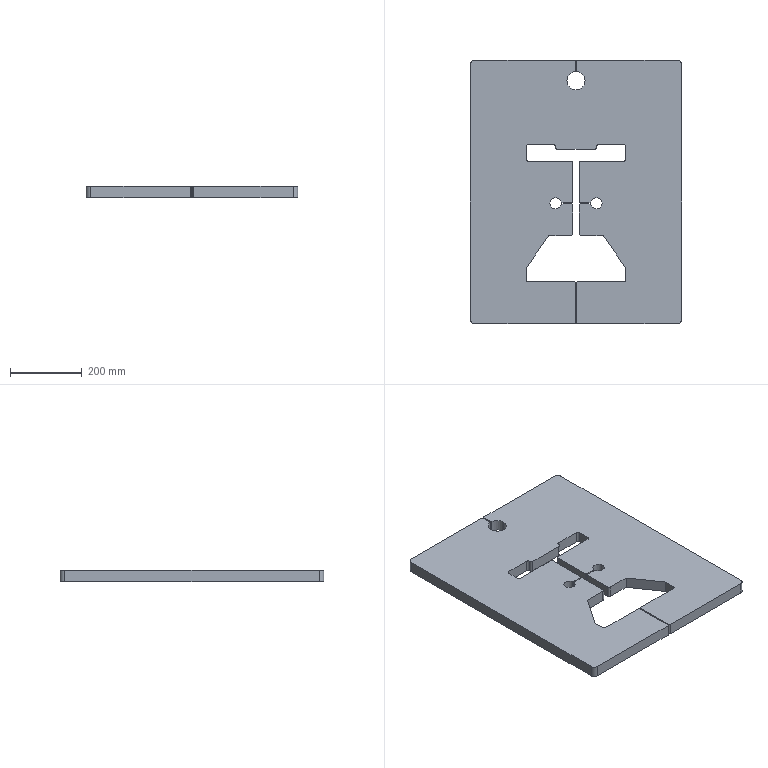Part | SolidWorks | features Extrusion 1 | 1 solid | 77 faces | box 591.82 x 736.6 x 32 mm | volume 12345944 mm3 | cylinder 40 | plane 37 | commonest cylinder face diameters 5 x16 11.6 x14 25.4 x4 31.75 x3 50.8 x3